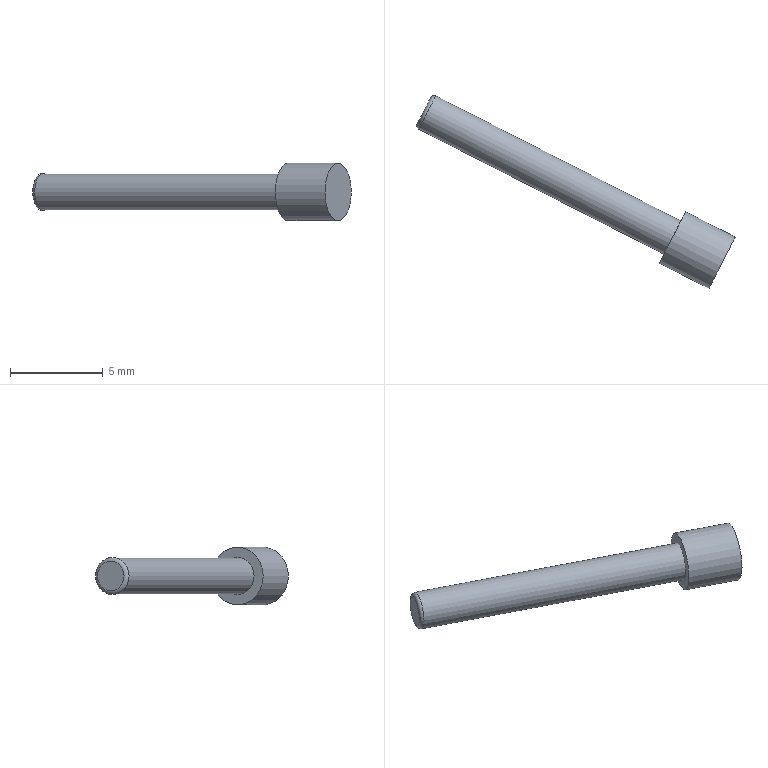Part | STEP file | gslz 2016.10.28-13_id74_x_t | 1 solid | 6 faces | box 17.127 x 10.375 x 3.1 mm | volume 69.715 mm3 | plane 3 | cylinder 2 | torus 1 | commonest cylinder face diameters 2 x1 3.1 x1
STEP:
#1=CARTESIAN_POINT('',(0.,0.,0.));
#2=DIRECTION('',(0.,0.,1.));
#3=DIRECTION('',(1.,0.,0.));
#4=AXIS2_PLACEMENT_3D('',#1,#2,#3);
#5=CARTESIAN_POINT('',(1091.745,-10.311,-19.491));
#6=VERTEX_POINT('',#5);
#7=CARTESIAN_POINT('',(1092.199,-9.42,-19.491));
#8=DIRECTION('',(0.891,-0.454,0.));
#9=DIRECTION('',(-0.454,-0.891,0.));
#10=AXIS2_PLACEMENT_3D('',#7,#8,#9);
#11=CIRCLE('',#10,1.);
#12=CARTESIAN_POINT('',(1092.021,-9.329,-19.491));
#13=DIRECTION('',(0.891,-0.454,0.));
#14=DIRECTION('',(0.454,0.891,0.));
#15=AXIS2_PLACEMENT_3D('',#12,#13,#14);
#16=CYLINDRICAL_SURFACE('',#15,1.);
#17=CARTESIAN_POINT('',(3.142,0.2));
#18=DIRECTION('',(1.,0.));
#19=VECTOR('',#18,1.);
#20=LINE('',#17,#19);
#21=(GEOMETRIC_REPRESENTATION_CONTEXT(2)PARAMETRIC_REPRESENTATION_CONTEXT()REPRESENTATION_CONTEXT('',''));
#22=DEFINITIONAL_REPRESENTATION('',(#20),#21);
#23=PCURVE('',#16,#22);
#24=CARTESIAN_POINT('',(1092.199,-9.42,-19.491));
#25=DIRECTION('',(-0.891,0.454,0.));
#26=DIRECTION('',(-0.454,-0.891,0.));
#27=AXIS2_PLACEMENT_3D('',#24,#25,#26);
#28=TOROIDAL_SURFACE('',#27,0.8,0.2);
#29=CARTESIAN_POINT('',(6.283,6.283));
#30=DIRECTION('',(-1.,0.));
#31=VECTOR('',#30,1.);
#32=LINE('',#29,#31);
#33=(GEOMETRIC_REPRESENTATION_CONTEXT(2)PARAMETRIC_REPRESENTATION_CONTEXT()REPRESENTATION_CONTEXT('',''));
#34=DEFINITIONAL_REPRESENTATION('',(#32),#33);
#35=PCURVE('',#28,#34);
#36=SURFACE_CURVE('',#11,(#23,#35),.PCURVE_S1.);
#37=EDGE_CURVE('',#6,#6,#36,.T.);
#38=ORIENTED_EDGE('',*,*,#37,.T.);
#39=CARTESIAN_POINT('',(1104.932,-17.03,-19.491));
#40=VERTEX_POINT('',#39);
#41=CARTESIAN_POINT('',(1091.745,-10.311,-19.491));
#42=CARTESIAN_POINT('',(1104.932,-17.03,-19.491));
#43=B_SPLINE_CURVE_WITH_KNOTS('',1,(#41,#42),.UNSPECIFIED.,.F.,.F.,(2,2),(0.2,15.),.PIECEWISE_BEZIER_KNOTS.);
#44=CARTESIAN_POINT('',(9.425,0.));
#45=DIRECTION('',(0.,1.));
#46=VECTOR('',#45,1.);
#47=LINE('',#44,#46);
#48=(GEOMETRIC_REPRESENTATION_CONTEXT(2)PARAMETRIC_REPRESENTATION_CONTEXT()REPRESENTATION_CONTEXT('',''));
#49=DEFINITIONAL_REPRESENTATION('',(#47),#48);
#50=PCURVE('',#16,#49);
#51=CARTESIAN_POINT('',(3.142,0.));
#52=DIRECTION('',(0.,1.));
#53=VECTOR('',#52,1.);
#54=LINE('',#51,#53);
#55=(GEOMETRIC_REPRESENTATION_CONTEXT(2)PARAMETRIC_REPRESENTATION_CONTEXT()REPRESENTATION_CONTEXT('',''));
#56=DEFINITIONAL_REPRESENTATION('',(#54),#55);
#57=PCURVE('',#16,#56);
#58=SEAM_CURVE('',#43,(#50,#57),.PCURVE_S1.);
#59=EDGE_CURVE('',#6,#40,#58,.T.);
#60=ORIENTED_EDGE('',*,*,#59,.T.);
#61=CARTESIAN_POINT('',(1105.386,-16.139,-19.491));
#62=DIRECTION('',(-0.891,0.454,0.));
#63=DIRECTION('',(-0.454,-0.891,0.));
#64=AXIS2_PLACEMENT_3D('',#61,#62,#63);
#65=CIRCLE('',#64,1.);
#66=CARTESIAN_POINT('',(9.425,15.));
#67=DIRECTION('',(-1.,0.));
#68=VECTOR('',#67,1.);
#69=LINE('',#66,#68);
#70=(GEOMETRIC_REPRESENTATION_CONTEXT(2)PARAMETRIC_REPRESENTATION_CONTEXT()REPRESENTATION_CONTEXT('',''));
#71=DEFINITIONAL_REPRESENTATION('',(#69),#70);
#72=PCURVE('',#16,#71);
#73=CARTESIAN_POINT('',(1105.386,-16.139,-19.491));
#74=DIRECTION('',(-0.891,0.454,0.));
#75=DIRECTION('',(-0.454,-0.891,0.));
#76=AXIS2_PLACEMENT_3D('',#73,#74,#75);
#77=PLANE('',#76);
#78=CARTESIAN_POINT('',(0.,0.));
#79=DIRECTION('',(1.,0.));
#80=AXIS2_PLACEMENT_2D('',#78,#79);
#81=CIRCLE('',#80,1.);
#82=(GEOMETRIC_REPRESENTATION_CONTEXT(2)PARAMETRIC_REPRESENTATION_CONTEXT()REPRESENTATION_CONTEXT('',''));
#83=DEFINITIONAL_REPRESENTATION('',(#81),#82);
#84=PCURVE('',#77,#83);
#85=SURFACE_CURVE('',#65,(#72,#84),.PCURVE_S1.);
#86=EDGE_CURVE('',#40,#40,#85,.T.);
#87=ORIENTED_EDGE('',*,*,#86,.T.);
#88=ORIENTED_EDGE('',*,*,#59,.F.);
#89=EDGE_LOOP('',(#38,#60,#87,#88));
#90=FACE_BOUND('',#89,.T.);
#91=ADVANCED_FACE('',(#90),#16,.T.);
#92=CARTESIAN_POINT('',(1091.658,-10.042,-19.491));
#93=VERTEX_POINT('',#92);
#94=CARTESIAN_POINT('',(1092.021,-9.329,-19.491));
#95=DIRECTION('',(-0.891,0.454,0.));
#96=DIRECTION('',(-0.454,-0.891,0.));
#97=AXIS2_PLACEMENT_3D('',#94,#95,#96);
#98=CIRCLE('',#97,0.8);
#99=CARTESIAN_POINT('',(1092.021,-9.329,-19.491));
#100=DIRECTION('',(-0.891,0.454,0.));
#101=DIRECTION('',(-0.454,-0.891,0.));
#102=AXIS2_PLACEMENT_3D('',#99,#100,#101);
#103=PLANE('',#102);
#104=CARTESIAN_POINT('',(0.,0.));
#105=DIRECTION('',(1.,0.));
#106=AXIS2_PLACEMENT_2D('',#104,#105);
#107=CIRCLE('',#106,0.8);
#108=(GEOMETRIC_REPRESENTATION_CONTEXT(2)PARAMETRIC_REPRESENTATION_CONTEXT()REPRESENTATION_CONTEXT('',''));
#109=DEFINITIONAL_REPRESENTATION('',(#107),#108);
#110=PCURVE('',#103,#109);
#111=CARTESIAN_POINT('',(0.,7.854));
#112=DIRECTION('',(1.,0.));
#113=VECTOR('',#112,1.);
#114=LINE('',#111,#113);
#115=(GEOMETRIC_REPRESENTATION_CONTEXT(2)PARAMETRIC_REPRESENTATION_CONTEXT()REPRESENTATION_CONTEXT('',''));
#116=DEFINITIONAL_REPRESENTATION('',(#114),#115);
#117=PCURVE('',#28,#116);
#118=SURFACE_CURVE('',#98,(#110,#117),.PCURVE_S1.);
#119=EDGE_CURVE('',#93,#93,#118,.T.);
#120=ORIENTED_EDGE('',*,*,#119,.T.);
#121=EDGE_LOOP('',(#120));
#122=FACE_BOUND('',#121,.T.);
#123=ADVANCED_FACE('',(#122),#103,.T.);
#124=ORIENTED_EDGE('',*,*,#37,.F.);
#125=CARTESIAN_POINT('',(1091.745,-10.311,-19.491));
#126=CARTESIAN_POINT('',(1091.698,-10.287,-19.491));
#127=CARTESIAN_POINT('',(1091.659,-10.248,-19.491));
#128=CARTESIAN_POINT('',(1091.634,-10.199,-19.491));
#129=CARTESIAN_POINT('',(1091.625,-10.144,-19.491));
#130=CARTESIAN_POINT('',(1091.634,-10.09,-19.491));
#131=CARTESIAN_POINT('',(1091.658,-10.042,-19.491));
#132=(BOUNDED_CURVE()B_SPLINE_CURVE(6,(#125,#126,#127,#128,#129,#130,#131),.UNSPECIFIED.,.F.,.F.)B_SPLINE_CURVE_WITH_KNOTS((7,7),(6.283,7.854),.PIECEWISE_BEZIER_KNOTS.)CURVE()GEOMETRIC_REPRESENTATION_ITEM()RATIONAL_B_SPLINE_CURVE((1.031,1.01,0.9979,0.994,0.9979,1.01,1.031))REPRESENTATION_ITEM(''));
#133=CARTESIAN_POINT('',(6.283,0.));
#134=DIRECTION('',(0.,1.));
#135=VECTOR('',#134,1.);
#136=LINE('',#133,#135);
#137=(GEOMETRIC_REPRESENTATION_CONTEXT(2)PARAMETRIC_REPRESENTATION_CONTEXT()REPRESENTATION_CONTEXT('',''));
#138=DEFINITIONAL_REPRESENTATION('',(#136),#137);
#139=PCURVE('',#28,#138);
#140=CARTESIAN_POINT('',(0.,0.));
#141=DIRECTION('',(0.,1.));
#142=VECTOR('',#141,1.);
#143=LINE('',#140,#142);
#144=(GEOMETRIC_REPRESENTATION_CONTEXT(2)PARAMETRIC_REPRESENTATION_CONTEXT()REPRESENTATION_CONTEXT('',''));
#145=DEFINITIONAL_REPRESENTATION('',(#143),#144);
#146=PCURVE('',#28,#145);
#147=SEAM_CURVE('',#132,(#139,#146),.PCURVE_S1.);
#148=EDGE_CURVE('',#6,#93,#147,.T.);
#149=ORIENTED_EDGE('',*,*,#148,.T.);
#150=ORIENTED_EDGE('',*,*,#119,.F.);
#151=ORIENTED_EDGE('',*,*,#148,.F.);
#152=EDGE_LOOP('',(#124,#149,#150,#151));
#153=FACE_BOUND('',#152,.T.);
#154=ADVANCED_FACE('',(#153),#28,.T.);
#155=CARTESIAN_POINT('',(1104.683,-17.52,-19.491));
#156=VERTEX_POINT('',#155);
#157=CARTESIAN_POINT('',(1105.386,-16.139,-19.491));
#158=DIRECTION('',(-0.891,0.454,0.));
#159=DIRECTION('',(-0.454,-0.891,0.));
#160=AXIS2_PLACEMENT_3D('',#157,#158,#159);
#161=CIRCLE('',#160,1.55);
#162=CARTESIAN_POINT('',(0.,0.));
#163=DIRECTION('',(1.,0.));
#164=AXIS2_PLACEMENT_2D('',#162,#163);
#165=CIRCLE('',#164,1.55);
#166=(GEOMETRIC_REPRESENTATION_CONTEXT(2)PARAMETRIC_REPRESENTATION_CONTEXT()REPRESENTATION_CONTEXT('',''));
#167=DEFINITIONAL_REPRESENTATION('',(#165),#166);
#168=PCURVE('',#77,#167);
#169=CARTESIAN_POINT('',(1108.059,-17.501,-19.491));
#170=DIRECTION('',(-0.891,0.454,0.));
#171=DIRECTION('',(-0.454,-0.891,0.));
#172=AXIS2_PLACEMENT_3D('',#169,#170,#171);
#173=CYLINDRICAL_SURFACE('',#172,1.55);
#174=CARTESIAN_POINT('',(0.,3.));
#175=DIRECTION('',(1.,0.));
#176=VECTOR('',#175,1.);
#177=LINE('',#174,#176);
#178=(GEOMETRIC_REPRESENTATION_CONTEXT(2)PARAMETRIC_REPRESENTATION_CONTEXT()REPRESENTATION_CONTEXT('',''));
#179=DEFINITIONAL_REPRESENTATION('',(#177),#178);
#180=PCURVE('',#173,#179);
#181=SURFACE_CURVE('',#161,(#168,#180),.PCURVE_S1.);
#182=EDGE_CURVE('',#156,#156,#181,.T.);
#183=ORIENTED_EDGE('',*,*,#182,.T.);
#184=EDGE_LOOP('',(#183));
#185=FACE_BOUND('',#184,.T.);
#186=ORIENTED_EDGE('',*,*,#86,.F.);
#187=EDGE_LOOP('',(#186));
#188=FACE_BOUND('',#187,.T.);
#189=ADVANCED_FACE('',(#185,#188),#77,.T.);
#190=CARTESIAN_POINT('',(1107.356,-18.882,-19.491));
#191=VERTEX_POINT('',#190);
#192=CARTESIAN_POINT('',(1108.059,-17.501,-19.491));
#193=DIRECTION('',(-0.891,0.454,0.));
#194=DIRECTION('',(-0.454,-0.891,0.));
#195=AXIS2_PLACEMENT_3D('',#192,#193,#194);
#196=CIRCLE('',#195,1.55);
#197=CARTESIAN_POINT('',(0.,0.));
#198=DIRECTION('',(1.,0.));
#199=VECTOR('',#198,1.);
#200=LINE('',#197,#199);
#201=(GEOMETRIC_REPRESENTATION_CONTEXT(2)PARAMETRIC_REPRESENTATION_CONTEXT()REPRESENTATION_CONTEXT('',''));
#202=DEFINITIONAL_REPRESENTATION('',(#200),#201);
#203=PCURVE('',#173,#202);
#204=CARTESIAN_POINT('',(1108.059,-17.501,-19.491));
#205=DIRECTION('',(-0.891,0.454,0.));
#206=DIRECTION('',(-0.454,-0.891,0.));
#207=AXIS2_PLACEMENT_3D('',#204,#205,#206);
#208=PLANE('',#207);
#209=CARTESIAN_POINT('',(0.,0.));
#210=DIRECTION('',(1.,0.));
#211=AXIS2_PLACEMENT_2D('',#209,#210);
#212=CIRCLE('',#211,1.55);
#213=(GEOMETRIC_REPRESENTATION_CONTEXT(2)PARAMETRIC_REPRESENTATION_CONTEXT()REPRESENTATION_CONTEXT('',''));
#214=DEFINITIONAL_REPRESENTATION('',(#212),#213);
#215=PCURVE('',#208,#214);
#216=SURFACE_CURVE('',#196,(#203,#215),.PCURVE_S1.);
#217=EDGE_CURVE('',#191,#191,#216,.T.);
#218=ORIENTED_EDGE('',*,*,#217,.T.);
#219=CARTESIAN_POINT('',(1107.356,-18.882,-19.491));
#220=CARTESIAN_POINT('',(1104.683,-17.52,-19.491));
#221=B_SPLINE_CURVE_WITH_KNOTS('',1,(#219,#220),.UNSPECIFIED.,.F.,.F.,(2,2),(0.,3.),.PIECEWISE_BEZIER_KNOTS.);
#222=CARTESIAN_POINT('',(6.283,0.));
#223=DIRECTION('',(0.,1.));
#224=VECTOR('',#223,1.);
#225=LINE('',#222,#224);
#226=(GEOMETRIC_REPRESENTATION_CONTEXT(2)PARAMETRIC_REPRESENTATION_CONTEXT()REPRESENTATION_CONTEXT('',''));
#227=DEFINITIONAL_REPRESENTATION('',(#225),#226);
#228=PCURVE('',#173,#227);
#229=CARTESIAN_POINT('',(0.,0.));
#230=DIRECTION('',(0.,1.));
#231=VECTOR('',#230,1.);
#232=LINE('',#229,#231);
#233=(GEOMETRIC_REPRESENTATION_CONTEXT(2)PARAMETRIC_REPRESENTATION_CONTEXT()REPRESENTATION_CONTEXT('',''));
#234=DEFINITIONAL_REPRESENTATION('',(#232),#233);
#235=PCURVE('',#173,#234);
#236=SEAM_CURVE('',#221,(#228,#235),.PCURVE_S1.);
#237=EDGE_CURVE('',#191,#156,#236,.T.);
#238=ORIENTED_EDGE('',*,*,#237,.T.);
#239=ORIENTED_EDGE('',*,*,#182,.F.);
#240=ORIENTED_EDGE('',*,*,#237,.F.);
#241=EDGE_LOOP('',(#218,#238,#239,#240));
#242=FACE_BOUND('',#241,.T.);
#243=ADVANCED_FACE('',(#242),#173,.T.);
#244=ORIENTED_EDGE('',*,*,#217,.F.);
#245=EDGE_LOOP('',(#244));
#246=FACE_BOUND('',#245,.T.);
#247=ADVANCED_FACE('',(#246),#208,.F.);
#248=CLOSED_SHELL('',(#91,#123,#154,#189,#243,#247));
#249=MANIFOLD_SOLID_BREP('',#248);
#250=(LENGTH_UNIT()NAMED_UNIT(*)SI_UNIT(.MILLI.,.METRE.));
#251=UNCERTAINTY_MEASURE_WITH_UNIT(LENGTH_MEASURE(0.00001),#250,'','');
#252=(NAMED_UNIT(*)PLANE_ANGLE_UNIT()SI_UNIT($,.RADIAN.));
#253=(NAMED_UNIT(*)SI_UNIT($,.STERADIAN.)SOLID_ANGLE_UNIT());
#254=(GEOMETRIC_REPRESENTATION_CONTEXT(3)GLOBAL_UNCERTAINTY_ASSIGNED_CONTEXT((#251))GLOBAL_UNIT_ASSIGNED_CONTEXT((#250,#252,#253))REPRESENTATION_CONTEXT('',''));
#255=ADVANCED_BREP_SHAPE_REPRESENTATION('',(#4,#249),#254);